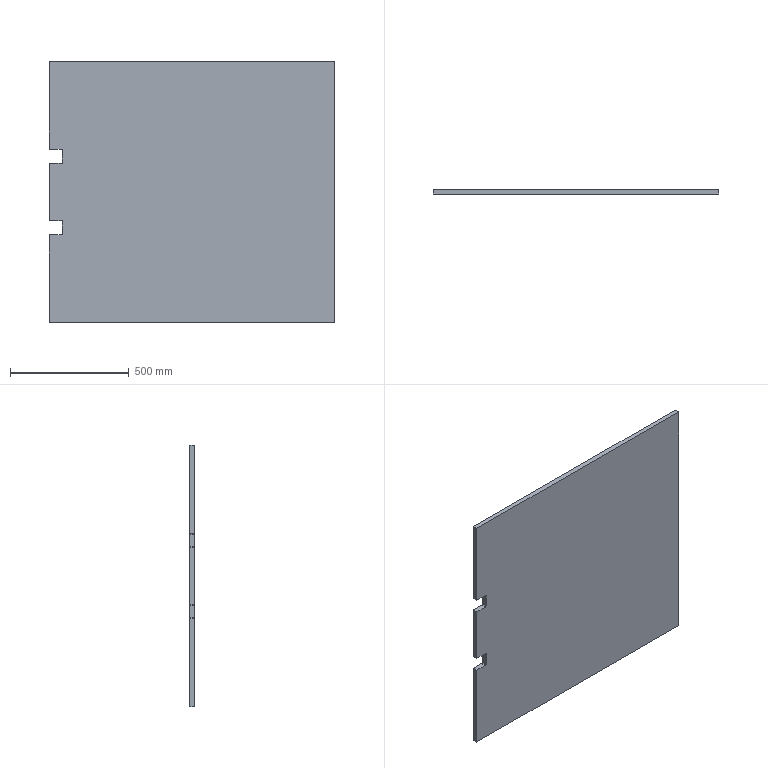Part | STEP file | A14-004 | 1 solid | 18 faces | box 1200 x 20 x 1100 mm | volume 26268429 mm3 | plane 14 | cylinder 4 | commonest cylinder face diameters 10 x4
STEP:
#1=CARTESIAN_POINT('',(0.,0.,0.));
#2=DIRECTION('',(0.,0.,1.));
#3=DIRECTION('',(1.,0.,0.));
#4=AXIS2_PLACEMENT_3D('',#1,#2,#3);
#5=CARTESIAN_POINT('',(-600.,0.,-120.));
#6=VERTEX_POINT('',#5);
#7=CARTESIAN_POINT('',(-600.,0.,120.));
#8=VERTEX_POINT('',#7);
#9=CARTESIAN_POINT('',(-600.,0.,-550.));
#10=DIRECTION('',(0.,0.,1.));
#11=VECTOR('',#10,1.);
#12=LINE('',#9,#11);
#13=CARTESIAN_POINT('',(-600.,20.,-550.));
#14=DIRECTION('',(1.,0.,0.));
#15=DIRECTION('',(0.,0.,-1.));
#16=AXIS2_PLACEMENT_3D('',#13,#14,#15);
#17=PLANE('',#16);
#18=CARTESIAN_POINT('',(0.,-20.));
#19=DIRECTION('',(-1.,0.));
#20=VECTOR('',#19,1.);
#21=LINE('',#18,#20);
#22=(GEOMETRIC_REPRESENTATION_CONTEXT(2)PARAMETRIC_REPRESENTATION_CONTEXT()REPRESENTATION_CONTEXT('',''));
#23=DEFINITIONAL_REPRESENTATION('',(#21),#22);
#24=PCURVE('',#17,#23);
#25=CARTESIAN_POINT('',(0.,0.,0.));
#26=DIRECTION('',(0.,1.,0.));
#27=DIRECTION('',(0.,0.,1.));
#28=AXIS2_PLACEMENT_3D('',#25,#26,#27);
#29=PLANE('',#28);
#30=CARTESIAN_POINT('',(-550.,-600.));
#31=DIRECTION('',(1.,0.));
#32=VECTOR('',#31,1.);
#33=LINE('',#30,#32);
#34=(GEOMETRIC_REPRESENTATION_CONTEXT(2)PARAMETRIC_REPRESENTATION_CONTEXT()REPRESENTATION_CONTEXT('',''));
#35=DEFINITIONAL_REPRESENTATION('',(#33),#34);
#36=PCURVE('',#29,#35);
#37=SURFACE_CURVE('',#12,(#24,#36),.PCURVE_S1.);
#38=EDGE_CURVE('',#6,#8,#37,.T.);
#39=ORIENTED_EDGE('',*,*,#38,.T.);
#40=CARTESIAN_POINT('',(-600.,20.,120.));
#41=VERTEX_POINT('',#40);
#42=CARTESIAN_POINT('',(-600.,0.,120.));
#43=DIRECTION('',(0.,1.,0.));
#44=VECTOR('',#43,1.);
#45=LINE('',#42,#44);
#46=CARTESIAN_POINT('',(-670.,-20.));
#47=DIRECTION('',(0.,1.));
#48=VECTOR('',#47,1.);
#49=LINE('',#46,#48);
#50=(GEOMETRIC_REPRESENTATION_CONTEXT(2)PARAMETRIC_REPRESENTATION_CONTEXT()REPRESENTATION_CONTEXT('',''));
#51=DEFINITIONAL_REPRESENTATION('',(#49),#50);
#52=PCURVE('',#17,#51);
#53=CARTESIAN_POINT('',(-600.,0.,120.));
#54=DIRECTION('',(0.,0.,-1.));
#55=DIRECTION('',(-1.,0.,0.));
#56=AXIS2_PLACEMENT_3D('',#53,#54,#55);
#57=PLANE('',#56);
#58=CARTESIAN_POINT('',(0.,0.));
#59=DIRECTION('',(0.,1.));
#60=VECTOR('',#59,1.);
#61=LINE('',#58,#60);
#62=(GEOMETRIC_REPRESENTATION_CONTEXT(2)PARAMETRIC_REPRESENTATION_CONTEXT()REPRESENTATION_CONTEXT('',''));
#63=DEFINITIONAL_REPRESENTATION('',(#61),#62);
#64=PCURVE('',#57,#63);
#65=SURFACE_CURVE('',#45,(#52,#64),.PCURVE_S1.);
#66=EDGE_CURVE('',#8,#41,#65,.T.);
#67=ORIENTED_EDGE('',*,*,#66,.T.);
#68=CARTESIAN_POINT('',(-600.,20.,-120.));
#69=VERTEX_POINT('',#68);
#70=CARTESIAN_POINT('',(-600.,20.,-550.));
#71=DIRECTION('',(0.,0.,1.));
#72=VECTOR('',#71,1.);
#73=LINE('',#70,#72);
#74=CARTESIAN_POINT('',(0.,0.));
#75=DIRECTION('',(-1.,0.));
#76=VECTOR('',#75,1.);
#77=LINE('',#74,#76);
#78=(GEOMETRIC_REPRESENTATION_CONTEXT(2)PARAMETRIC_REPRESENTATION_CONTEXT()REPRESENTATION_CONTEXT('',''));
#79=DEFINITIONAL_REPRESENTATION('',(#77),#78);
#80=PCURVE('',#17,#79);
#81=CARTESIAN_POINT('',(0.,20.,0.));
#82=DIRECTION('',(0.,1.,0.));
#83=DIRECTION('',(0.,0.,1.));
#84=AXIS2_PLACEMENT_3D('',#81,#82,#83);
#85=PLANE('',#84);
#86=CARTESIAN_POINT('',(-550.,-600.));
#87=DIRECTION('',(1.,0.));
#88=VECTOR('',#87,1.);
#89=LINE('',#86,#88);
#90=(GEOMETRIC_REPRESENTATION_CONTEXT(2)PARAMETRIC_REPRESENTATION_CONTEXT()REPRESENTATION_CONTEXT('',''));
#91=DEFINITIONAL_REPRESENTATION('',(#89),#90);
#92=PCURVE('',#85,#91);
#93=SURFACE_CURVE('',#73,(#80,#92),.PCURVE_S1.);
#94=EDGE_CURVE('',#69,#41,#93,.T.);
#95=ORIENTED_EDGE('',*,*,#94,.F.);
#96=CARTESIAN_POINT('',(-600.,0.,-120.));
#97=DIRECTION('',(0.,1.,0.));
#98=VECTOR('',#97,1.);
#99=LINE('',#96,#98);
#100=CARTESIAN_POINT('',(-430.,-20.));
#101=DIRECTION('',(0.,1.));
#102=VECTOR('',#101,1.);
#103=LINE('',#100,#102);
#104=(GEOMETRIC_REPRESENTATION_CONTEXT(2)PARAMETRIC_REPRESENTATION_CONTEXT()REPRESENTATION_CONTEXT('',''));
#105=DEFINITIONAL_REPRESENTATION('',(#103),#104);
#106=PCURVE('',#17,#105);
#107=CARTESIAN_POINT('',(-600.,0.,-120.));
#108=DIRECTION('',(0.,0.,1.));
#109=DIRECTION('',(1.,0.,0.));
#110=AXIS2_PLACEMENT_3D('',#107,#108,#109);
#111=PLANE('',#110);
#112=CARTESIAN_POINT('',(0.,0.));
#113=DIRECTION('',(0.,1.));
#114=VECTOR('',#113,1.);
#115=LINE('',#112,#114);
#116=(GEOMETRIC_REPRESENTATION_CONTEXT(2)PARAMETRIC_REPRESENTATION_CONTEXT()REPRESENTATION_CONTEXT('',''));
#117=DEFINITIONAL_REPRESENTATION('',(#115),#116);
#118=PCURVE('',#111,#117);
#119=SURFACE_CURVE('',#99,(#106,#118),.PCURVE_S1.);
#120=EDGE_CURVE('',#6,#69,#119,.T.);
#121=ORIENTED_EDGE('',*,*,#120,.F.);
#122=EDGE_LOOP('',(#39,#67,#95,#121));
#123=FACE_BOUND('',#122,.T.);
#124=ADVANCED_FACE('',(#123),#17,.F.);
#125=CARTESIAN_POINT('',(-600.,0.,-550.));
#126=VERTEX_POINT('',#125);
#127=CARTESIAN_POINT('',(-600.,0.,-180.));
#128=VERTEX_POINT('',#127);
#129=CARTESIAN_POINT('',(-600.,0.,-550.));
#130=DIRECTION('',(0.,0.,1.));
#131=VECTOR('',#130,1.);
#132=LINE('',#129,#131);
#133=CARTESIAN_POINT('',(-600.,20.,-550.));
#134=DIRECTION('',(1.,0.,0.));
#135=DIRECTION('',(0.,0.,-1.));
#136=AXIS2_PLACEMENT_3D('',#133,#134,#135);
#137=PLANE('',#136);
#138=CARTESIAN_POINT('',(0.,-20.));
#139=DIRECTION('',(-1.,0.));
#140=VECTOR('',#139,1.);
#141=LINE('',#138,#140);
#142=(GEOMETRIC_REPRESENTATION_CONTEXT(2)PARAMETRIC_REPRESENTATION_CONTEXT()REPRESENTATION_CONTEXT('',''));
#143=DEFINITIONAL_REPRESENTATION('',(#141),#142);
#144=PCURVE('',#137,#143);
#145=CARTESIAN_POINT('',(-550.,-600.));
#146=DIRECTION('',(1.,0.));
#147=VECTOR('',#146,1.);
#148=LINE('',#145,#147);
#149=(GEOMETRIC_REPRESENTATION_CONTEXT(2)PARAMETRIC_REPRESENTATION_CONTEXT()REPRESENTATION_CONTEXT('',''));
#150=DEFINITIONAL_REPRESENTATION('',(#148),#149);
#151=PCURVE('',#29,#150);
#152=SURFACE_CURVE('',#132,(#144,#151),.PCURVE_S1.);
#153=EDGE_CURVE('',#126,#128,#152,.T.);
#154=ORIENTED_EDGE('',*,*,#153,.T.);
#155=CARTESIAN_POINT('',(-600.,20.,-180.));
#156=VERTEX_POINT('',#155);
#157=CARTESIAN_POINT('',(-600.,0.,-180.));
#158=DIRECTION('',(0.,1.,0.));
#159=VECTOR('',#158,1.);
#160=LINE('',#157,#159);
#161=CARTESIAN_POINT('',(-370.,-20.));
#162=DIRECTION('',(0.,1.));
#163=VECTOR('',#162,1.);
#164=LINE('',#161,#163);
#165=(GEOMETRIC_REPRESENTATION_CONTEXT(2)PARAMETRIC_REPRESENTATION_CONTEXT()REPRESENTATION_CONTEXT('',''));
#166=DEFINITIONAL_REPRESENTATION('',(#164),#165);
#167=PCURVE('',#137,#166);
#168=CARTESIAN_POINT('',(-600.,0.,-180.));
#169=DIRECTION('',(0.,0.,-1.));
#170=DIRECTION('',(-1.,0.,0.));
#171=AXIS2_PLACEMENT_3D('',#168,#169,#170);
#172=PLANE('',#171);
#173=CARTESIAN_POINT('',(0.,0.));
#174=DIRECTION('',(0.,1.));
#175=VECTOR('',#174,1.);
#176=LINE('',#173,#175);
#177=(GEOMETRIC_REPRESENTATION_CONTEXT(2)PARAMETRIC_REPRESENTATION_CONTEXT()REPRESENTATION_CONTEXT('',''));
#178=DEFINITIONAL_REPRESENTATION('',(#176),#177);
#179=PCURVE('',#172,#178);
#180=SURFACE_CURVE('',#160,(#167,#179),.PCURVE_S1.);
#181=EDGE_CURVE('',#128,#156,#180,.T.);
#182=ORIENTED_EDGE('',*,*,#181,.T.);
#183=CARTESIAN_POINT('',(-600.,20.,-550.));
#184=VERTEX_POINT('',#183);
#185=CARTESIAN_POINT('',(-600.,20.,-550.));
#186=DIRECTION('',(0.,0.,1.));
#187=VECTOR('',#186,1.);
#188=LINE('',#185,#187);
#189=CARTESIAN_POINT('',(0.,0.));
#190=DIRECTION('',(-1.,0.));
#191=VECTOR('',#190,1.);
#192=LINE('',#189,#191);
#193=(GEOMETRIC_REPRESENTATION_CONTEXT(2)PARAMETRIC_REPRESENTATION_CONTEXT()REPRESENTATION_CONTEXT('',''));
#194=DEFINITIONAL_REPRESENTATION('',(#192),#193);
#195=PCURVE('',#137,#194);
#196=CARTESIAN_POINT('',(-550.,-600.));
#197=DIRECTION('',(1.,0.));
#198=VECTOR('',#197,1.);
#199=LINE('',#196,#198);
#200=(GEOMETRIC_REPRESENTATION_CONTEXT(2)PARAMETRIC_REPRESENTATION_CONTEXT()REPRESENTATION_CONTEXT('',''));
#201=DEFINITIONAL_REPRESENTATION('',(#199),#200);
#202=PCURVE('',#85,#201);
#203=SURFACE_CURVE('',#188,(#195,#202),.PCURVE_S1.);
#204=EDGE_CURVE('',#184,#156,#203,.T.);
#205=ORIENTED_EDGE('',*,*,#204,.F.);
#206=CARTESIAN_POINT('',(-600.,20.,-550.));
#207=DIRECTION('',(0.,-1.,0.));
#208=VECTOR('',#207,1.);
#209=LINE('',#206,#208);
#210=CARTESIAN_POINT('',(0.,0.));
#211=DIRECTION('',(0.,-1.));
#212=VECTOR('',#211,1.);
#213=LINE('',#210,#212);
#214=(GEOMETRIC_REPRESENTATION_CONTEXT(2)PARAMETRIC_REPRESENTATION_CONTEXT()REPRESENTATION_CONTEXT('',''));
#215=DEFINITIONAL_REPRESENTATION('',(#213),#214);
#216=PCURVE('',#137,#215);
#217=CARTESIAN_POINT('',(-600.,20.,-550.));
#218=DIRECTION('',(0.,0.,1.));
#219=DIRECTION('',(1.,0.,0.));
#220=AXIS2_PLACEMENT_3D('',#217,#218,#219);
#221=PLANE('',#220);
#222=CARTESIAN_POINT('',(0.,0.));
#223=DIRECTION('',(0.,-1.));
#224=VECTOR('',#223,1.);
#225=LINE('',#222,#224);
#226=(GEOMETRIC_REPRESENTATION_CONTEXT(2)PARAMETRIC_REPRESENTATION_CONTEXT()REPRESENTATION_CONTEXT('',''));
#227=DEFINITIONAL_REPRESENTATION('',(#225),#226);
#228=PCURVE('',#221,#227);
#229=SURFACE_CURVE('',#209,(#216,#228),.PCURVE_S1.);
#230=EDGE_CURVE('',#184,#126,#229,.T.);
#231=ORIENTED_EDGE('',*,*,#230,.T.);
#232=EDGE_LOOP('',(#154,#182,#205,#231));
#233=FACE_BOUND('',#232,.T.);
#234=ADVANCED_FACE('',(#233),#137,.F.);
#235=CARTESIAN_POINT('',(600.,0.,550.));
#236=VERTEX_POINT('',#235);
#237=CARTESIAN_POINT('',(600.,0.,-550.));
#238=VERTEX_POINT('',#237);
#239=CARTESIAN_POINT('',(600.,0.,-550.));
#240=DIRECTION('',(0.,0.,-1.));
#241=VECTOR('',#240,1.);
#242=LINE('',#239,#241);
#243=CARTESIAN_POINT('',(600.,20.,-550.));
#244=DIRECTION('',(-1.,0.,0.));
#245=DIRECTION('',(0.,0.,1.));
#246=AXIS2_PLACEMENT_3D('',#243,#244,#245);
#247=PLANE('',#246);
#248=CARTESIAN_POINT('',(0.,-20.));
#249=DIRECTION('',(-1.,0.));
#250=VECTOR('',#249,1.);
#251=LINE('',#248,#250);
#252=(GEOMETRIC_REPRESENTATION_CONTEXT(2)PARAMETRIC_REPRESENTATION_CONTEXT()REPRESENTATION_CONTEXT('',''));
#253=DEFINITIONAL_REPRESENTATION('',(#251),#252);
#254=PCURVE('',#247,#253);
#255=CARTESIAN_POINT('',(-550.,600.));
#256=DIRECTION('',(-1.,0.));
#257=VECTOR('',#256,1.);
#258=LINE('',#255,#257);
#259=(GEOMETRIC_REPRESENTATION_CONTEXT(2)PARAMETRIC_REPRESENTATION_CONTEXT()REPRESENTATION_CONTEXT('',''));
#260=DEFINITIONAL_REPRESENTATION('',(#258),#259);
#261=PCURVE('',#29,#260);
#262=SURFACE_CURVE('',#242,(#254,#261),.PCURVE_S1.);
#263=EDGE_CURVE('',#236,#238,#262,.T.);
#264=ORIENTED_EDGE('',*,*,#263,.T.);
#265=CARTESIAN_POINT('',(600.,20.,-550.));
#266=VERTEX_POINT('',#265);
#267=CARTESIAN_POINT('',(600.,20.,-550.));
#268=DIRECTION('',(0.,-1.,0.));
#269=VECTOR('',#268,1.);
#270=LINE('',#267,#269);
#271=CARTESIAN_POINT('',(0.,0.));
#272=DIRECTION('',(0.,-1.));
#273=VECTOR('',#272,1.);
#274=LINE('',#271,#273);
#275=(GEOMETRIC_REPRESENTATION_CONTEXT(2)PARAMETRIC_REPRESENTATION_CONTEXT()REPRESENTATION_CONTEXT('',''));
#276=DEFINITIONAL_REPRESENTATION('',(#274),#275);
#277=PCURVE('',#247,#276);
#278=CARTESIAN_POINT('',(1200.,0.));
#279=DIRECTION('',(0.,-1.));
#280=VECTOR('',#279,1.);
#281=LINE('',#278,#280);
#282=(GEOMETRIC_REPRESENTATION_CONTEXT(2)PARAMETRIC_REPRESENTATION_CONTEXT()REPRESENTATION_CONTEXT('',''));
#283=DEFINITIONAL_REPRESENTATION('',(#281),#282);
#284=PCURVE('',#221,#283);
#285=SURFACE_CURVE('',#270,(#277,#284),.PCURVE_S1.);
#286=EDGE_CURVE('',#266,#238,#285,.T.);
#287=ORIENTED_EDGE('',*,*,#286,.F.);
#288=CARTESIAN_POINT('',(600.,20.,550.));
#289=VERTEX_POINT('',#288);
#290=CARTESIAN_POINT('',(600.,20.,-550.));
#291=DIRECTION('',(0.,0.,-1.));
#292=VECTOR('',#291,1.);
#293=LINE('',#290,#292);
#294=CARTESIAN_POINT('',(0.,0.));
#295=DIRECTION('',(-1.,0.));
#296=VECTOR('',#295,1.);
#297=LINE('',#294,#296);
#298=(GEOMETRIC_REPRESENTATION_CONTEXT(2)PARAMETRIC_REPRESENTATION_CONTEXT()REPRESENTATION_CONTEXT('',''));
#299=DEFINITIONAL_REPRESENTATION('',(#297),#298);
#300=PCURVE('',#247,#299);
#301=CARTESIAN_POINT('',(-550.,600.));
#302=DIRECTION('',(-1.,0.));
#303=VECTOR('',#302,1.);
#304=LINE('',#301,#303);
#305=(GEOMETRIC_REPRESENTATION_CONTEXT(2)PARAMETRIC_REPRESENTATION_CONTEXT()REPRESENTATION_CONTEXT('',''));
#306=DEFINITIONAL_REPRESENTATION('',(#304),#305);
#307=PCURVE('',#85,#306);
#308=SURFACE_CURVE('',#293,(#300,#307),.PCURVE_S1.);
#309=EDGE_CURVE('',#289,#266,#308,.T.);
#310=ORIENTED_EDGE('',*,*,#309,.F.);
#311=CARTESIAN_POINT('',(600.,20.,550.));
#312=DIRECTION('',(0.,-1.,0.));
#313=VECTOR('',#312,1.);
#314=LINE('',#311,#313);
#315=CARTESIAN_POINT('',(1100.,0.));
#316=DIRECTION('',(0.,-1.));
#317=VECTOR('',#316,1.);
#318=LINE('',#315,#317);
#319=(GEOMETRIC_REPRESENTATION_CONTEXT(2)PARAMETRIC_REPRESENTATION_CONTEXT()REPRESENTATION_CONTEXT('',''));
#320=DEFINITIONAL_REPRESENTATION('',(#318),#319);
#321=PCURVE('',#247,#320);
#322=CARTESIAN_POINT('',(-600.,20.,550.));
#323=DIRECTION('',(0.,0.,-1.));
#324=DIRECTION('',(-1.,0.,0.));
#325=AXIS2_PLACEMENT_3D('',#322,#323,#324);
#326=PLANE('',#325);
#327=CARTESIAN_POINT('',(-1200.,0.));
#328=DIRECTION('',(0.,-1.));
#329=VECTOR('',#328,1.);
#330=LINE('',#327,#329);
#331=(GEOMETRIC_REPRESENTATION_CONTEXT(2)PARAMETRIC_REPRESENTATION_CONTEXT()REPRESENTATION_CONTEXT('',''));
#332=DEFINITIONAL_REPRESENTATION('',(#330),#331);
#333=PCURVE('',#326,#332);
#334=SURFACE_CURVE('',#314,(#321,#333),.PCURVE_S1.);
#335=EDGE_CURVE('',#289,#236,#334,.T.);
#336=ORIENTED_EDGE('',*,*,#335,.T.);
#337=EDGE_LOOP('',(#264,#287,#310,#336));
#338=FACE_BOUND('',#337,.T.);
#339=ADVANCED_FACE('',(#338),#247,.F.);
#340=CARTESIAN_POINT('',(-600.,0.,-550.));
#341=DIRECTION('',(-1.,0.,0.));
#342=VECTOR('',#341,1.);
#343=LINE('',#340,#342);
#344=CARTESIAN_POINT('',(0.,-20.));
#345=DIRECTION('',(-1.,0.));
#346=VECTOR('',#345,1.);
#347=LINE('',#344,#346);
#348=(GEOMETRIC_REPRESENTATION_CONTEXT(2)PARAMETRIC_REPRESENTATION_CONTEXT()REPRESENTATION_CONTEXT('',''));
#349=DEFINITIONAL_REPRESENTATION('',(#347),#348);
#350=PCURVE('',#221,#349);
#351=CARTESIAN_POINT('',(-550.,-600.));
#352=DIRECTION('',(0.,-1.));
#353=VECTOR('',#352,1.);
#354=LINE('',#351,#353);
#355=(GEOMETRIC_REPRESENTATION_CONTEXT(2)PARAMETRIC_REPRESENTATION_CONTEXT()REPRESENTATION_CONTEXT('',''));
#356=DEFINITIONAL_REPRESENTATION('',(#354),#355);
#357=PCURVE('',#29,#356);
#358=SURFACE_CURVE('',#343,(#350,#357),.PCURVE_S1.);
#359=EDGE_CURVE('',#238,#126,#358,.T.);
#360=ORIENTED_EDGE('',*,*,#359,.T.);
#361=ORIENTED_EDGE('',*,*,#230,.F.);
#362=CARTESIAN_POINT('',(-600.,20.,-550.));
#363=DIRECTION('',(-1.,0.,0.));
#364=VECTOR('',#363,1.);
#365=LINE('',#362,#364);
#366=CARTESIAN_POINT('',(0.,0.));
#367=DIRECTION('',(-1.,0.));
#368=VECTOR('',#367,1.);
#369=LINE('',#366,#368);
#370=(GEOMETRIC_REPRESENTATION_CONTEXT(2)PARAMETRIC_REPRESENTATION_CONTEXT()REPRESENTATION_CONTEXT('',''));
#371=DEFINITIONAL_REPRESENTATION('',(#369),#370);
#372=PCURVE('',#221,#371);
#373=CARTESIAN_POINT('',(-550.,-600.));
#374=DIRECTION('',(0.,-1.));
#375=VECTOR('',#374,1.);
#376=LINE('',#373,#375);
#377=(GEOMETRIC_REPRESENTATION_CONTEXT(2)PARAMETRIC_REPRESENTATION_CONTEXT()REPRESENTATION_CONTEXT('',''));
#378=DEFINITIONAL_REPRESENTATION('',(#376),#377);
#379=PCURVE('',#85,#378);
#380=SURFACE_CURVE('',#365,(#372,#379),.PCURVE_S1.);
#381=EDGE_CURVE('',#266,#184,#380,.T.);
#382=ORIENTED_EDGE('',*,*,#381,.F.);
#383=ORIENTED_EDGE('',*,*,#286,.T.);
#384=EDGE_LOOP('',(#360,#361,#382,#383));
#385=FACE_BOUND('',#384,.T.);
#386=ADVANCED_FACE('',(#385),#221,.F.);
#387=CARTESIAN_POINT('',(-600.,20.,180.));
#388=VERTEX_POINT('',#387);
#389=CARTESIAN_POINT('',(-600.,20.,550.));
#390=VERTEX_POINT('',#389);
#391=CARTESIAN_POINT('',(-600.,20.,-550.));
#392=DIRECTION('',(0.,0.,1.));
#393=VECTOR('',#392,1.);
#394=LINE('',#391,#393);
#395=CARTESIAN_POINT('',(-600.,20.,-550.));
#396=DIRECTION('',(1.,0.,0.));
#397=DIRECTION('',(0.,0.,-1.));
#398=AXIS2_PLACEMENT_3D('',#395,#396,#397);
#399=PLANE('',#398);
#400=CARTESIAN_POINT('',(0.,0.));
#401=DIRECTION('',(-1.,0.));
#402=VECTOR('',#401,1.);
#403=LINE('',#400,#402);
#404=(GEOMETRIC_REPRESENTATION_CONTEXT(2)PARAMETRIC_REPRESENTATION_CONTEXT()REPRESENTATION_CONTEXT('',''));
#405=DEFINITIONAL_REPRESENTATION('',(#403),#404);
#406=PCURVE('',#399,#405);
#407=CARTESIAN_POINT('',(-550.,-600.));
#408=DIRECTION('',(1.,0.));
#409=VECTOR('',#408,1.);
#410=LINE('',#407,#409);
#411=(GEOMETRIC_REPRESENTATION_CONTEXT(2)PARAMETRIC_REPRESENTATION_CONTEXT()REPRESENTATION_CONTEXT('',''));
#412=DEFINITIONAL_REPRESENTATION('',(#410),#411);
#413=PCURVE('',#85,#412);
#414=SURFACE_CURVE('',#394,(#406,#413),.PCURVE_S1.);
#415=EDGE_CURVE('',#388,#390,#414,.T.);
#416=ORIENTED_EDGE('',*,*,#415,.F.);
#417=CARTESIAN_POINT('',(-600.,0.,180.));
#418=VERTEX_POINT('',#417);
#419=CARTESIAN_POINT('',(-600.,0.,180.));
#420=DIRECTION('',(0.,1.,0.));
#421=VECTOR('',#420,1.);
#422=LINE('',#419,#421);
#423=CARTESIAN_POINT('',(-730.,-20.));
#424=DIRECTION('',(0.,1.));
#425=VECTOR('',#424,1.);
#426=LINE('',#423,#425);
#427=(GEOMETRIC_REPRESENTATION_CONTEXT(2)PARAMETRIC_REPRESENTATION_CONTEXT()REPRESENTATION_CONTEXT('',''));
#428=DEFINITIONAL_REPRESENTATION('',(#426),#427);
#429=PCURVE('',#399,#428);
#430=CARTESIAN_POINT('',(-600.,0.,180.));
#431=DIRECTION('',(0.,0.,1.));
#432=DIRECTION('',(1.,0.,0.));
#433=AXIS2_PLACEMENT_3D('',#430,#431,#432);
#434=PLANE('',#433);
#435=CARTESIAN_POINT('',(0.,0.));
#436=DIRECTION('',(0.,1.));
#437=VECTOR('',#436,1.);
#438=LINE('',#435,#437);
#439=(GEOMETRIC_REPRESENTATION_CONTEXT(2)PARAMETRIC_REPRESENTATION_CONTEXT()REPRESENTATION_CONTEXT('',''));
#440=DEFINITIONAL_REPRESENTATION('',(#438),#439);
#441=PCURVE('',#434,#440);
#442=SURFACE_CURVE('',#422,(#429,#441),.PCURVE_S1.);
#443=EDGE_CURVE('',#418,#388,#442,.T.);
#444=ORIENTED_EDGE('',*,*,#443,.F.);
#445=CARTESIAN_POINT('',(-600.,0.,550.));
#446=VERTEX_POINT('',#445);
#447=CARTESIAN_POINT('',(-600.,0.,-550.));
#448=DIRECTION('',(0.,0.,1.));
#449=VECTOR('',#448,1.);
#450=LINE('',#447,#449);
#451=CARTESIAN_POINT('',(0.,-20.));
#452=DIRECTION('',(-1.,0.));
#453=VECTOR('',#452,1.);
#454=LINE('',#451,#453);
#455=(GEOMETRIC_REPRESENTATION_CONTEXT(2)PARAMETRIC_REPRESENTATION_CONTEXT()REPRESENTATION_CONTEXT('',''));
#456=DEFINITIONAL_REPRESENTATION('',(#454),#455);
#457=PCURVE('',#399,#456);
#458=CARTESIAN_POINT('',(-550.,-600.));
#459=DIRECTION('',(1.,0.));
#460=VECTOR('',#459,1.);
#461=LINE('',#458,#460);
#462=(GEOMETRIC_REPRESENTATION_CONTEXT(2)PARAMETRIC_REPRESENTATION_CONTEXT()REPRESENTATION_CONTEXT('',''));
#463=DEFINITIONAL_REPRESENTATION('',(#461),#462);
#464=PCURVE('',#29,#463);
#465=SURFACE_CURVE('',#450,(#457,#464),.PCURVE_S1.);
#466=EDGE_CURVE('',#418,#446,#465,.T.);
#467=ORIENTED_EDGE('',*,*,#466,.T.);
#468=CARTESIAN_POINT('',(-600.,20.,550.));
#469=DIRECTION('',(0.,-1.,0.));
#470=VECTOR('',#469,1.);
#471=LINE('',#468,#470);
#472=CARTESIAN_POINT('',(-1100.,0.));
#473=DIRECTION('',(0.,-1.));
#474=VECTOR('',#473,1.);
#475=LINE('',#472,#474);
#476=(GEOMETRIC_REPRESENTATION_CONTEXT(2)PARAMETRIC_REPRESENTATION_CONTEXT()REPRESENTATION_CONTEXT('',''));
#477=DEFINITIONAL_REPRESENTATION('',(#475),#476);
#478=PCURVE('',#399,#477);
#479=CARTESIAN_POINT('',(0.,0.));
#480=DIRECTION('',(0.,-1.));
#481=VECTOR('',#480,1.);
#482=LINE('',#479,#481);
#483=(GEOMETRIC_REPRESENTATION_CONTEXT(2)PARAMETRIC_REPRESENTATION_CONTEXT()REPRESENTATION_CONTEXT('',''));
#484=DEFINITIONAL_REPRESENTATION('',(#482),#483);
#485=PCURVE('',#326,#484);
#486=SURFACE_CURVE('',#471,(#478,#485),.PCURVE_S1.);
#487=EDGE_CURVE('',#390,#446,#486,.T.);
#488=ORIENTED_EDGE('',*,*,#487,.F.);
#489=EDGE_LOOP('',(#416,#444,#467,#488));
#490=FACE_BOUND('',#489,.T.);
#491=ADVANCED_FACE('',(#490),#399,.F.);
#492=CARTESIAN_POINT('',(-600.,0.,550.));
#493=DIRECTION('',(1.,0.,0.));
#494=VECTOR('',#493,1.);
#495=LINE('',#492,#494);
#496=CARTESIAN_POINT('',(0.,-20.));
#497=DIRECTION('',(-1.,0.));
#498=VECTOR('',#497,1.);
#499=LINE('',#496,#498);
#500=(GEOMETRIC_REPRESENTATION_CONTEXT(2)PARAMETRIC_REPRESENTATION_CONTEXT()REPRESENTATION_CONTEXT('',''));
#501=DEFINITIONAL_REPRESENTATION('',(#499),#500);
#502=PCURVE('',#326,#501);
#503=CARTESIAN_POINT('',(550.,-600.));
#504=DIRECTION('',(0.,1.));
#505=VECTOR('',#504,1.);
#506=LINE('',#503,#505);
#507=(GEOMETRIC_REPRESENTATION_CONTEXT(2)PARAMETRIC_REPRESENTATION_CONTEXT()REPRESENTATION_CONTEXT('',''));
#508=DEFINITIONAL_REPRESENTATION('',(#506),#507);
#509=PCURVE('',#29,#508);
#510=SURFACE_CURVE('',#495,(#502,#509),.PCURVE_S1.);
#511=EDGE_CURVE('',#446,#236,#510,.T.);
#512=ORIENTED_EDGE('',*,*,#511,.T.);
#513=ORIENTED_EDGE('',*,*,#335,.F.);
#514=CARTESIAN_POINT('',(-600.,20.,550.));
#515=DIRECTION('',(1.,0.,0.));
#516=VECTOR('',#515,1.);
#517=LINE('',#514,#516);
#518=CARTESIAN_POINT('',(0.,0.));
#519=DIRECTION('',(-1.,0.));
#520=VECTOR('',#519,1.);
#521=LINE('',#518,#520);
#522=(GEOMETRIC_REPRESENTATION_CONTEXT(2)PARAMETRIC_REPRESENTATION_CONTEXT()REPRESENTATION_CONTEXT('',''));
#523=DEFINITIONAL_REPRESENTATION('',(#521),#522);
#524=PCURVE('',#326,#523);
#525=CARTESIAN_POINT('',(550.,-600.));
#526=DIRECTION('',(0.,1.));
#527=VECTOR('',#526,1.);
#528=LINE('',#525,#527);
#529=(GEOMETRIC_REPRESENTATION_CONTEXT(2)PARAMETRIC_REPRESENTATION_CONTEXT()REPRESENTATION_CONTEXT('',''));
#530=DEFINITIONAL_REPRESENTATION('',(#528),#529);
#531=PCURVE('',#85,#530);
#532=SURFACE_CURVE('',#517,(#524,#531),.PCURVE_S1.);
#533=EDGE_CURVE('',#390,#289,#532,.T.);
#534=ORIENTED_EDGE('',*,*,#533,.F.);
#535=ORIENTED_EDGE('',*,*,#487,.T.);
#536=EDGE_LOOP('',(#512,#513,#534,#535));
#537=FACE_BOUND('',#536,.T.);
#538=ADVANCED_FACE('',(#537),#326,.F.);
#539=CARTESIAN_POINT('',(-550.,20.,120.));
#540=VERTEX_POINT('',#539);
#541=CARTESIAN_POINT('',(-600.,20.,120.));
#542=DIRECTION('',(-1.,0.,0.));
#543=VECTOR('',#542,1.);
#544=LINE('',#541,#543);
#545=CARTESIAN_POINT('',(120.,-600.));
#546=DIRECTION('',(0.,-1.));
#547=VECTOR('',#546,1.);
#548=LINE('',#545,#547);
#549=(GEOMETRIC_REPRESENTATION_CONTEXT(2)PARAMETRIC_REPRESENTATION_CONTEXT()REPRESENTATION_CONTEXT('',''));
#550=DEFINITIONAL_REPRESENTATION('',(#548),#549);
#551=PCURVE('',#85,#550);
#552=CARTESIAN_POINT('',(0.,20.));
#553=DIRECTION('',(1.,0.));
#554=VECTOR('',#553,1.);
#555=LINE('',#552,#554);
#556=(GEOMETRIC_REPRESENTATION_CONTEXT(2)PARAMETRIC_REPRESENTATION_CONTEXT()REPRESENTATION_CONTEXT('',''));
#557=DEFINITIONAL_REPRESENTATION('',(#555),#556);
#558=PCURVE('',#57,#557);
#559=SURFACE_CURVE('',#544,(#551,#558),.PCURVE_S1.);
#560=EDGE_CURVE('',#540,#41,#559,.T.);
#561=ORIENTED_EDGE('',*,*,#560,.F.);
#562=CARTESIAN_POINT('',(-545.,20.,125.));
#563=VERTEX_POINT('',#562);
#564=CARTESIAN_POINT('',(-550.,20.,125.));
#565=DIRECTION('',(0.,1.,0.));
#566=DIRECTION('',(0.,0.,-1.));
#567=AXIS2_PLACEMENT_3D('',#564,#565,#566);
#568=CIRCLE('',#567,5.);
#569=CARTESIAN_POINT('',(125.,-550.));
#570=DIRECTION('',(-1.,0.));
#571=AXIS2_PLACEMENT_2D('',#569,#570);
#572=CIRCLE('',#571,5.);
#573=(GEOMETRIC_REPRESENTATION_CONTEXT(2)PARAMETRIC_REPRESENTATION_CONTEXT()REPRESENTATION_CONTEXT('',''));
#574=DEFINITIONAL_REPRESENTATION('',(#572),#573);
#575=PCURVE('',#85,#574);
#576=CARTESIAN_POINT('',(-550.,0.,125.));
#577=DIRECTION('',(0.,1.,0.));
#578=DIRECTION('',(0.,0.,1.));
#579=AXIS2_PLACEMENT_3D('',#576,#577,#578);
#580=CYLINDRICAL_SURFACE('',#579,5.);
#581=CARTESIAN_POINT('',(-3.142,20.));
#582=DIRECTION('',(1.,0.));
#583=VECTOR('',#582,1.);
#584=LINE('',#581,#583);
#585=(GEOMETRIC_REPRESENTATION_CONTEXT(2)PARAMETRIC_REPRESENTATION_CONTEXT()REPRESENTATION_CONTEXT('',''));
#586=DEFINITIONAL_REPRESENTATION('',(#584),#585);
#587=PCURVE('',#580,#586);
#588=SURFACE_CURVE('',#568,(#575,#587),.PCURVE_S1.);
#589=EDGE_CURVE('',#563,#540,#588,.T.);
#590=ORIENTED_EDGE('',*,*,#589,.F.);
#591=CARTESIAN_POINT('',(-545.,20.,175.));
#592=VERTEX_POINT('',#591);
#593=CARTESIAN_POINT('',(-545.,20.,175.));
#594=DIRECTION('',(0.,0.,-1.));
#595=VECTOR('',#594,1.);
#596=LINE('',#593,#595);
#597=CARTESIAN_POINT('',(175.,-545.));
#598=DIRECTION('',(-1.,0.));
#599=VECTOR('',#598,1.);
#600=LINE('',#597,#599);
#601=(GEOMETRIC_REPRESENTATION_CONTEXT(2)PARAMETRIC_REPRESENTATION_CONTEXT()REPRESENTATION_CONTEXT('',''));
#602=DEFINITIONAL_REPRESENTATION('',(#600),#601);
#603=PCURVE('',#85,#602);
#604=CARTESIAN_POINT('',(-545.,0.,175.));
#605=DIRECTION('',(1.,0.,0.));
#606=DIRECTION('',(0.,0.,-1.));
#607=AXIS2_PLACEMENT_3D('',#604,#605,#606);
#608=PLANE('',#607);
#609=CARTESIAN_POINT('',(0.,20.));
#610=DIRECTION('',(1.,0.));
#611=VECTOR('',#610,1.);
#612=LINE('',#609,#611);
#613=(GEOMETRIC_REPRESENTATION_CONTEXT(2)PARAMETRIC_REPRESENTATION_CONTEXT()REPRESENTATION_CONTEXT('',''));
#614=DEFINITIONAL_REPRESENTATION('',(#612),#613);
#615=PCURVE('',#608,#614);
#616=SURFACE_CURVE('',#596,(#603,#615),.PCURVE_S1.);
#617=EDGE_CURVE('',#592,#563,#616,.T.);
#618=ORIENTED_EDGE('',*,*,#617,.F.);
#619=CARTESIAN_POINT('',(-550.,20.,180.));
#620=VERTEX_POINT('',#619);
#621=CARTESIAN_POINT('',(-550.,20.,175.));
#622=DIRECTION('',(0.,1.,0.));
#623=DIRECTION('',(0.,0.,1.));
#624=AXIS2_PLACEMENT_3D('',#621,#622,#623);
#625=CIRCLE('',#624,5.);
#626=CARTESIAN_POINT('',(175.,-550.));
#627=DIRECTION('',(1.,0.));
#628=AXIS2_PLACEMENT_2D('',#626,#627);
#629=CIRCLE('',#628,5.);
#630=(GEOMETRIC_REPRESENTATION_CONTEXT(2)PARAMETRIC_REPRESENTATION_CONTEXT()REPRESENTATION_CONTEXT('',''));
#631=DEFINITIONAL_REPRESENTATION('',(#629),#630);
#632=PCURVE('',#85,#631);
#633=CARTESIAN_POINT('',(-550.,0.,175.));
#634=DIRECTION('',(0.,1.,0.));
#635=DIRECTION('',(0.,0.,1.));
#636=AXIS2_PLACEMENT_3D('',#633,#634,#635);
#637=CYLINDRICAL_SURFACE('',#636,5.);
#638=CARTESIAN_POINT('',(0.,20.));
#639=DIRECTION('',(1.,0.));
#640=VECTOR('',#639,1.);
#641=LINE('',#638,#640);
#642=(GEOMETRIC_REPRESENTATION_CONTEXT(2)PARAMETRIC_REPRESENTATION_CONTEXT()REPRESENTATION_CONTEXT('',''));
#643=DEFINITIONAL_REPRESENTATION('',(#641),#642);
#644=PCURVE('',#637,#643);
#645=SURFACE_CURVE('',#625,(#632,#644),.PCURVE_S1.);
#646=EDGE_CURVE('',#620,#592,#645,.T.);
#647=ORIENTED_EDGE('',*,*,#646,.F.);
#648=CARTESIAN_POINT('',(-600.,20.,180.));
#649=DIRECTION('',(1.,0.,0.));
#650=VECTOR('',#649,1.);
#651=LINE('',#648,#650);
#652=CARTESIAN_POINT('',(180.,-600.));
#653=DIRECTION('',(0.,1.));
#654=VECTOR('',#653,1.);
#655=LINE('',#652,#654);
#656=(GEOMETRIC_REPRESENTATION_CONTEXT(2)PARAMETRIC_REPRESENTATION_CONTEXT()REPRESENTATION_CONTEXT('',''));
#657=DEFINITIONAL_REPRESENTATION('',(#655),#656);
#658=PCURVE('',#85,#657);
#659=CARTESIAN_POINT('',(0.,20.));
#660=DIRECTION('',(1.,0.));
#661=VECTOR('',#660,1.);
#662=LINE('',#659,#661);
#663=(GEOMETRIC_REPRESENTATION_CONTEXT(2)PARAMETRIC_REPRESENTATION_CONTEXT()REPRESENTATION_CONTEXT('',''));
#664=DEFINITIONAL_REPRESENTATION('',(#662),#663);
#665=PCURVE('',#434,#664);
#666=SURFACE_CURVE('',#651,(#658,#665),.PCURVE_S1.);
#667=EDGE_CURVE('',#388,#620,#666,.T.);
#668=ORIENTED_EDGE('',*,*,#667,.F.);
#669=ORIENTED_EDGE('',*,*,#415,.T.);
#670=ORIENTED_EDGE('',*,*,#533,.T.);
#671=ORIENTED_EDGE('',*,*,#309,.T.);
#672=ORIENTED_EDGE('',*,*,#381,.T.);
#673=ORIENTED_EDGE('',*,*,#204,.T.);
#674=CARTESIAN_POINT('',(-550.,20.,-180.));
#675=VERTEX_POINT('',#674);
#676=CARTESIAN_POINT('',(-600.,20.,-180.));
#677=DIRECTION('',(-1.,0.,0.));
#678=VECTOR('',#677,1.);
#679=LINE('',#676,#678);
#680=CARTESIAN_POINT('',(-180.,-600.));
#681=DIRECTION('',(0.,-1.));
#682=VECTOR('',#681,1.);
#683=LINE('',#680,#682);
#684=(GEOMETRIC_REPRESENTATION_CONTEXT(2)PARAMETRIC_REPRESENTATION_CONTEXT()REPRESENTATION_CONTEXT('',''));
#685=DEFINITIONAL_REPRESENTATION('',(#683),#684);
#686=PCURVE('',#85,#685);
#687=CARTESIAN_POINT('',(0.,20.));
#688=DIRECTION('',(1.,0.));
#689=VECTOR('',#688,1.);
#690=LINE('',#687,#689);
#691=(GEOMETRIC_REPRESENTATION_CONTEXT(2)PARAMETRIC_REPRESENTATION_CONTEXT()REPRESENTATION_CONTEXT('',''));
#692=DEFINITIONAL_REPRESENTATION('',(#690),#691);
#693=PCURVE('',#172,#692);
#694=SURFACE_CURVE('',#679,(#686,#693),.PCURVE_S1.);
#695=EDGE_CURVE('',#675,#156,#694,.T.);
#696=ORIENTED_EDGE('',*,*,#695,.F.);
#697=CARTESIAN_POINT('',(-545.,20.,-175.));
#698=VERTEX_POINT('',#697);
#699=CARTESIAN_POINT('',(-550.,20.,-175.));
#700=DIRECTION('',(0.,1.,0.));
#701=DIRECTION('',(0.,0.,-1.));
#702=AXIS2_PLACEMENT_3D('',#699,#700,#701);
#703=CIRCLE('',#702,5.);
#704=CARTESIAN_POINT('',(-175.,-550.));
#705=DIRECTION('',(-1.,0.));
#706=AXIS2_PLACEMENT_2D('',#704,#705);
#707=CIRCLE('',#706,5.);
#708=(GEOMETRIC_REPRESENTATION_CONTEXT(2)PARAMETRIC_REPRESENTATION_CONTEXT()REPRESENTATION_CONTEXT('',''));
#709=DEFINITIONAL_REPRESENTATION('',(#707),#708);
#710=PCURVE('',#85,#709);
#711=CARTESIAN_POINT('',(-550.,0.,-175.));
#712=DIRECTION('',(0.,1.,0.));
#713=DIRECTION('',(0.,0.,1.));
#714=AXIS2_PLACEMENT_3D('',#711,#712,#713);
#715=CYLINDRICAL_SURFACE('',#714,5.);
#716=CARTESIAN_POINT('',(-3.142,20.));
#717=DIRECTION('',(1.,0.));
#718=VECTOR('',#717,1.);
#719=LINE('',#716,#718);
#720=(GEOMETRIC_REPRESENTATION_CONTEXT(2)PARAMETRIC_REPRESENTATION_CONTEXT()REPRESENTATION_CONTEXT('',''));
#721=DEFINITIONAL_REPRESENTATION('',(#719),#720);
#722=PCURVE('',#715,#721);
#723=SURFACE_CURVE('',#703,(#710,#722),.PCURVE_S1.);
#724=EDGE_CURVE('',#698,#675,#723,.T.);
#725=ORIENTED_EDGE('',*,*,#724,.F.);
#726=CARTESIAN_POINT('',(-545.,20.,-125.));
#727=VERTEX_POINT('',#726);
#728=CARTESIAN_POINT('',(-545.,20.,-175.));
#729=DIRECTION('',(0.,0.,-1.));
#730=VECTOR('',#729,1.);
#731=LINE('',#728,#730);
#732=CARTESIAN_POINT('',(-175.,-545.));
#733=DIRECTION('',(-1.,0.));
#734=VECTOR('',#733,1.);
#735=LINE('',#732,#734);
#736=(GEOMETRIC_REPRESENTATION_CONTEXT(2)PARAMETRIC_REPRESENTATION_CONTEXT()REPRESENTATION_CONTEXT('',''));
#737=DEFINITIONAL_REPRESENTATION('',(#735),#736);
#738=PCURVE('',#85,#737);
#739=CARTESIAN_POINT('',(-545.,0.,-175.));
#740=DIRECTION('',(1.,0.,0.));
#741=DIRECTION('',(0.,0.,-1.));
#742=AXIS2_PLACEMENT_3D('',#739,#740,#741);
#743=PLANE('',#742);
#744=CARTESIAN_POINT('',(0.,20.));
#745=DIRECTION('',(1.,0.));
#746=VECTOR('',#745,1.);
#747=LINE('',#744,#746);
#748=(GEOMETRIC_REPRESENTATION_CONTEXT(2)PARAMETRIC_REPRESENTATION_CONTEXT()REPRESENTATION_CONTEXT('',''));
#749=DEFINITIONAL_REPRESENTATION('',(#747),#748);
#750=PCURVE('',#743,#749);
#751=SURFACE_CURVE('',#731,(#738,#750),.PCURVE_S1.);
#752=EDGE_CURVE('',#727,#698,#751,.T.);
#753=ORIENTED_EDGE('',*,*,#752,.F.);
#754=CARTESIAN_POINT('',(-550.,20.,-120.));
#755=VERTEX_POINT('',#754);
#756=CARTESIAN_POINT('',(-550.,20.,-125.));
#757=DIRECTION('',(0.,1.,0.));
#758=DIRECTION('',(0.,0.,1.));
#759=AXIS2_PLACEMENT_3D('',#756,#757,#758);
#760=CIRCLE('',#759,5.);
#761=CARTESIAN_POINT('',(-125.,-550.));
#762=DIRECTION('',(1.,0.));
#763=AXIS2_PLACEMENT_2D('',#761,#762);
#764=CIRCLE('',#763,5.);
#765=(GEOMETRIC_REPRESENTATION_CONTEXT(2)PARAMETRIC_REPRESENTATION_CONTEXT()REPRESENTATION_CONTEXT('',''));
#766=DEFINITIONAL_REPRESENTATION('',(#764),#765);
#767=PCURVE('',#85,#766);
#768=CARTESIAN_POINT('',(-550.,0.,-125.));
#769=DIRECTION('',(0.,1.,0.));
#770=DIRECTION('',(0.,0.,1.));
#771=AXIS2_PLACEMENT_3D('',#768,#769,#770);
#772=CYLINDRICAL_SURFACE('',#771,5.);
#773=CARTESIAN_POINT('',(0.,20.));
#774=DIRECTION('',(1.,0.));
#775=VECTOR('',#774,1.);
#776=LINE('',#773,#775);
#777=(GEOMETRIC_REPRESENTATION_CONTEXT(2)PARAMETRIC_REPRESENTATION_CONTEXT()REPRESENTATION_CONTEXT('',''));
#778=DEFINITIONAL_REPRESENTATION('',(#776),#777);
#779=PCURVE('',#772,#778);
#780=SURFACE_CURVE('',#760,(#767,#779),.PCURVE_S1.);
#781=EDGE_CURVE('',#755,#727,#780,.T.);
#782=ORIENTED_EDGE('',*,*,#781,.F.);
#783=CARTESIAN_POINT('',(-600.,20.,-120.));
#784=DIRECTION('',(1.,0.,0.));
#785=VECTOR('',#784,1.);
#786=LINE('',#783,#785);
#787=CARTESIAN_POINT('',(-120.,-600.));
#788=DIRECTION('',(0.,1.));
#789=VECTOR('',#788,1.);
#790=LINE('',#787,#789);
#791=(GEOMETRIC_REPRESENTATION_CONTEXT(2)PARAMETRIC_REPRESENTATION_CONTEXT()REPRESENTATION_CONTEXT('',''));
#792=DEFINITIONAL_REPRESENTATION('',(#790),#791);
#793=PCURVE('',#85,#792);
#794=CARTESIAN_POINT('',(0.,20.));
#795=DIRECTION('',(1.,0.));
#796=VECTOR('',#795,1.);
#797=LINE('',#794,#796);
#798=(GEOMETRIC_REPRESENTATION_CONTEXT(2)PARAMETRIC_REPRESENTATION_CONTEXT()REPRESENTATION_CONTEXT('',''));
#799=DEFINITIONAL_REPRESENTATION('',(#797),#798);
#800=PCURVE('',#111,#799);
#801=SURFACE_CURVE('',#786,(#793,#800),.PCURVE_S1.);
#802=EDGE_CURVE('',#69,#755,#801,.T.);
#803=ORIENTED_EDGE('',*,*,#802,.F.);
#804=ORIENTED_EDGE('',*,*,#94,.T.);
#805=EDGE_LOOP('',(#561,#590,#618,#647,#668,#669,#670,#671,#672,#673,#696,#725,#753,#782,#803,#804));
#806=FACE_BOUND('',#805,.T.);
#807=ADVANCED_FACE('',(#806),#85,.T.);
#808=CARTESIAN_POINT('',(-545.,0.,125.));
#809=VERTEX_POINT('',#808);
#810=CARTESIAN_POINT('',(-550.,0.,120.));
#811=VERTEX_POINT('',#810);
#812=CARTESIAN_POINT('',(-550.,0.,125.));
#813=DIRECTION('',(0.,1.,0.));
#814=DIRECTION('',(0.,0.,-1.));
#815=AXIS2_PLACEMENT_3D('',#812,#813,#814);
#816=CIRCLE('',#815,5.);
#817=CARTESIAN_POINT('',(125.,-550.));
#818=DIRECTION('',(-1.,0.));
#819=AXIS2_PLACEMENT_2D('',#817,#818);
#820=CIRCLE('',#819,5.);
#821=(GEOMETRIC_REPRESENTATION_CONTEXT(2)PARAMETRIC_REPRESENTATION_CONTEXT()REPRESENTATION_CONTEXT('',''));
#822=DEFINITIONAL_REPRESENTATION('',(#820),#821);
#823=PCURVE('',#29,#822);
#824=CARTESIAN_POINT('',(-3.142,0.));
#825=DIRECTION('',(1.,0.));
#826=VECTOR('',#825,1.);
#827=LINE('',#824,#826);
#828=(GEOMETRIC_REPRESENTATION_CONTEXT(2)PARAMETRIC_REPRESENTATION_CONTEXT()REPRESENTATION_CONTEXT('',''));
#829=DEFINITIONAL_REPRESENTATION('',(#827),#828);
#830=PCURVE('',#580,#829);
#831=SURFACE_CURVE('',#816,(#823,#830),.PCURVE_S1.);
#832=EDGE_CURVE('',#809,#811,#831,.T.);
#833=ORIENTED_EDGE('',*,*,#832,.T.);
#834=CARTESIAN_POINT('',(-600.,0.,120.));
#835=DIRECTION('',(-1.,0.,0.));
#836=VECTOR('',#835,1.);
#837=LINE('',#834,#836);
#838=CARTESIAN_POINT('',(120.,-600.));
#839=DIRECTION('',(0.,-1.));
#840=VECTOR('',#839,1.);
#841=LINE('',#838,#840);
#842=(GEOMETRIC_REPRESENTATION_CONTEXT(2)PARAMETRIC_REPRESENTATION_CONTEXT()REPRESENTATION_CONTEXT('',''));
#843=DEFINITIONAL_REPRESENTATION('',(#841),#842);
#844=PCURVE('',#29,#843);
#845=CARTESIAN_POINT('',(0.,0.));
#846=DIRECTION('',(1.,0.));
#847=VECTOR('',#846,1.);
#848=LINE('',#845,#847);
#849=(GEOMETRIC_REPRESENTATION_CONTEXT(2)PARAMETRIC_REPRESENTATION_CONTEXT()REPRESENTATION_CONTEXT('',''));
#850=DEFINITIONAL_REPRESENTATION('',(#848),#849);
#851=PCURVE('',#57,#850);
#852=SURFACE_CURVE('',#837,(#844,#851),.PCURVE_S1.);
#853=EDGE_CURVE('',#811,#8,#852,.T.);
#854=ORIENTED_EDGE('',*,*,#853,.T.);
#855=ORIENTED_EDGE('',*,*,#38,.F.);
#856=CARTESIAN_POINT('',(-550.,0.,-120.));
#857=VERTEX_POINT('',#856);
#858=CARTESIAN_POINT('',(-600.,0.,-120.));
#859=DIRECTION('',(1.,0.,0.));
#860=VECTOR('',#859,1.);
#861=LINE('',#858,#860);
#862=CARTESIAN_POINT('',(-120.,-600.));
#863=DIRECTION('',(0.,1.));
#864=VECTOR('',#863,1.);
#865=LINE('',#862,#864);
#866=(GEOMETRIC_REPRESENTATION_CONTEXT(2)PARAMETRIC_REPRESENTATION_CONTEXT()REPRESENTATION_CONTEXT('',''));
#867=DEFINITIONAL_REPRESENTATION('',(#865),#866);
#868=PCURVE('',#29,#867);
#869=CARTESIAN_POINT('',(0.,0.));
#870=DIRECTION('',(1.,0.));
#871=VECTOR('',#870,1.);
#872=LINE('',#869,#871);
#873=(GEOMETRIC_REPRESENTATION_CONTEXT(2)PARAMETRIC_REPRESENTATION_CONTEXT()REPRESENTATION_CONTEXT('',''));
#874=DEFINITIONAL_REPRESENTATION('',(#872),#873);
#875=PCURVE('',#111,#874);
#876=SURFACE_CURVE('',#861,(#868,#875),.PCURVE_S1.);
#877=EDGE_CURVE('',#6,#857,#876,.T.);
#878=ORIENTED_EDGE('',*,*,#877,.T.);
#879=CARTESIAN_POINT('',(-545.,0.,-125.));
#880=VERTEX_POINT('',#879);
#881=CARTESIAN_POINT('',(-550.,0.,-125.));
#882=DIRECTION('',(0.,1.,0.));
#883=DIRECTION('',(0.,0.,1.));
#884=AXIS2_PLACEMENT_3D('',#881,#882,#883);
#885=CIRCLE('',#884,5.);
#886=CARTESIAN_POINT('',(-125.,-550.));
#887=DIRECTION('',(1.,0.));
#888=AXIS2_PLACEMENT_2D('',#886,#887);
#889=CIRCLE('',#888,5.);
#890=(GEOMETRIC_REPRESENTATION_CONTEXT(2)PARAMETRIC_REPRESENTATION_CONTEXT()REPRESENTATION_CONTEXT('',''));
#891=DEFINITIONAL_REPRESENTATION('',(#889),#890);
#892=PCURVE('',#29,#891);
#893=CARTESIAN_POINT('',(0.,0.));
#894=DIRECTION('',(1.,0.));
#895=VECTOR('',#894,1.);
#896=LINE('',#893,#895);
#897=(GEOMETRIC_REPRESENTATION_CONTEXT(2)PARAMETRIC_REPRESENTATION_CONTEXT()REPRESENTATION_CONTEXT('',''));
#898=DEFINITIONAL_REPRESENTATION('',(#896),#897);
#899=PCURVE('',#772,#898);
#900=SURFACE_CURVE('',#885,(#892,#899),.PCURVE_S1.);
#901=EDGE_CURVE('',#857,#880,#900,.T.);
#902=ORIENTED_EDGE('',*,*,#901,.T.);
#903=CARTESIAN_POINT('',(-545.,0.,-175.));
#904=VERTEX_POINT('',#903);
#905=CARTESIAN_POINT('',(-545.,0.,-175.));
#906=DIRECTION('',(0.,0.,-1.));
#907=VECTOR('',#906,1.);
#908=LINE('',#905,#907);
#909=CARTESIAN_POINT('',(-175.,-545.));
#910=DIRECTION('',(-1.,0.));
#911=VECTOR('',#910,1.);
#912=LINE('',#909,#911);
#913=(GEOMETRIC_REPRESENTATION_CONTEXT(2)PARAMETRIC_REPRESENTATION_CONTEXT()REPRESENTATION_CONTEXT('',''));
#914=DEFINITIONAL_REPRESENTATION('',(#912),#913);
#915=PCURVE('',#29,#914);
#916=CARTESIAN_POINT('',(0.,0.));
#917=DIRECTION('',(1.,0.));
#918=VECTOR('',#917,1.);
#919=LINE('',#916,#918);
#920=(GEOMETRIC_REPRESENTATION_CONTEXT(2)PARAMETRIC_REPRESENTATION_CONTEXT()REPRESENTATION_CONTEXT('',''));
#921=DEFINITIONAL_REPRESENTATION('',(#919),#920);
#922=PCURVE('',#743,#921);
#923=SURFACE_CURVE('',#908,(#915,#922),.PCURVE_S1.);
#924=EDGE_CURVE('',#880,#904,#923,.T.);
#925=ORIENTED_EDGE('',*,*,#924,.T.);
#926=CARTESIAN_POINT('',(-550.,0.,-180.));
#927=VERTEX_POINT('',#926);
#928=CARTESIAN_POINT('',(-550.,0.,-175.));
#929=DIRECTION('',(0.,1.,0.));
#930=DIRECTION('',(0.,0.,-1.));
#931=AXIS2_PLACEMENT_3D('',#928,#929,#930);
#932=CIRCLE('',#931,5.);
#933=CARTESIAN_POINT('',(-175.,-550.));
#934=DIRECTION('',(-1.,0.));
#935=AXIS2_PLACEMENT_2D('',#933,#934);
#936=CIRCLE('',#935,5.);
#937=(GEOMETRIC_REPRESENTATION_CONTEXT(2)PARAMETRIC_REPRESENTATION_CONTEXT()REPRESENTATION_CONTEXT('',''));
#938=DEFINITIONAL_REPRESENTATION('',(#936),#937);
#939=PCURVE('',#29,#938);
#940=CARTESIAN_POINT('',(-3.142,0.));
#941=DIRECTION('',(1.,0.));
#942=VECTOR('',#941,1.);
#943=LINE('',#940,#942);
#944=(GEOMETRIC_REPRESENTATION_CONTEXT(2)PARAMETRIC_REPRESENTATION_CONTEXT()REPRESENTATION_CONTEXT('',''));
#945=DEFINITIONAL_REPRESENTATION('',(#943),#944);
#946=PCURVE('',#715,#945);
#947=SURFACE_CURVE('',#932,(#939,#946),.PCURVE_S1.);
#948=EDGE_CURVE('',#904,#927,#947,.T.);
#949=ORIENTED_EDGE('',*,*,#948,.T.);
#950=CARTESIAN_POINT('',(-600.,0.,-180.));
#951=DIRECTION('',(-1.,0.,0.));
#952=VECTOR('',#951,1.);
#953=LINE('',#950,#952);
#954=CARTESIAN_POINT('',(-180.,-600.));
#955=DIRECTION('',(0.,-1.));
#956=VECTOR('',#955,1.);
#957=LINE('',#954,#956);
#958=(GEOMETRIC_REPRESENTATION_CONTEXT(2)PARAMETRIC_REPRESENTATION_CONTEXT()REPRESENTATION_CONTEXT('',''));
#959=DEFINITIONAL_REPRESENTATION('',(#957),#958);
#960=PCURVE('',#29,#959);
#961=CARTESIAN_POINT('',(0.,0.));
#962=DIRECTION('',(1.,0.));
#963=VECTOR('',#962,1.);
#964=LINE('',#961,#963);
#965=(GEOMETRIC_REPRESENTATION_CONTEXT(2)PARAMETRIC_REPRESENTATION_CONTEXT()REPRESENTATION_CONTEXT('',''));
#966=DEFINITIONAL_REPRESENTATION('',(#964),#965);
#967=PCURVE('',#172,#966);
#968=SURFACE_CURVE('',#953,(#960,#967),.PCURVE_S1.);
#969=EDGE_CURVE('',#927,#128,#968,.T.);
#970=ORIENTED_EDGE('',*,*,#969,.T.);
#971=ORIENTED_EDGE('',*,*,#153,.F.);
#972=ORIENTED_EDGE('',*,*,#359,.F.);
#973=ORIENTED_EDGE('',*,*,#263,.F.);
#974=ORIENTED_EDGE('',*,*,#511,.F.);
#975=ORIENTED_EDGE('',*,*,#466,.F.);
#976=CARTESIAN_POINT('',(-550.,0.,180.));
#977=VERTEX_POINT('',#976);
#978=CARTESIAN_POINT('',(-600.,0.,180.));
#979=DIRECTION('',(1.,0.,0.));
#980=VECTOR('',#979,1.);
#981=LINE('',#978,#980);
#982=CARTESIAN_POINT('',(180.,-600.));
#983=DIRECTION('',(0.,1.));
#984=VECTOR('',#983,1.);
#985=LINE('',#982,#984);
#986=(GEOMETRIC_REPRESENTATION_CONTEXT(2)PARAMETRIC_REPRESENTATION_CONTEXT()REPRESENTATION_CONTEXT('',''));
#987=DEFINITIONAL_REPRESENTATION('',(#985),#986);
#988=PCURVE('',#29,#987);
#989=CARTESIAN_POINT('',(0.,0.));
#990=DIRECTION('',(1.,0.));
#991=VECTOR('',#990,1.);
#992=LINE('',#989,#991);
#993=(GEOMETRIC_REPRESENTATION_CONTEXT(2)PARAMETRIC_REPRESENTATION_CONTEXT()REPRESENTATION_CONTEXT('',''));
#994=DEFINITIONAL_REPRESENTATION('',(#992),#993);
#995=PCURVE('',#434,#994);
#996=SURFACE_CURVE('',#981,(#988,#995),.PCURVE_S1.);
#997=EDGE_CURVE('',#418,#977,#996,.T.);
#998=ORIENTED_EDGE('',*,*,#997,.T.);
#999=CARTESIAN_POINT('',(-545.,0.,175.));
#1000=VERTEX_POINT('',#999);
#1001=CARTESIAN_POINT('',(-550.,0.,175.));
#1002=DIRECTION('',(0.,1.,0.));
#1003=DIRECTION('',(0.,0.,1.));
#1004=AXIS2_PLACEMENT_3D('',#1001,#1002,#1003);
#1005=CIRCLE('',#1004,5.);
#1006=CARTESIAN_POINT('',(175.,-550.));
#1007=DIRECTION('',(1.,0.));
#1008=AXIS2_PLACEMENT_2D('',#1006,#1007);
#1009=CIRCLE('',#1008,5.);
#1010=(GEOMETRIC_REPRESENTATION_CONTEXT(2)PARAMETRIC_REPRESENTATION_CONTEXT()REPRESENTATION_CONTEXT('',''));
#1011=DEFINITIONAL_REPRESENTATION('',(#1009),#1010);
#1012=PCURVE('',#29,#1011);
#1013=CARTESIAN_POINT('',(0.,0.));
#1014=DIRECTION('',(1.,0.));
#1015=VECTOR('',#1014,1.);
#1016=LINE('',#1013,#1015);
#1017=(GEOMETRIC_REPRESENTATION_CONTEXT(2)PARAMETRIC_REPRESENTATION_CONTEXT()REPRESENTATION_CONTEXT('',''));
#1018=DEFINITIONAL_REPRESENTATION('',(#1016),#1017);
#1019=PCURVE('',#637,#1018);
#1020=SURFACE_CURVE('',#1005,(#1012,#1019),.PCURVE_S1.);
#1021=EDGE_CURVE('',#977,#1000,#1020,.T.);
#1022=ORIENTED_EDGE('',*,*,#1021,.T.);
#1023=CARTESIAN_POINT('',(-545.,0.,175.));
#1024=DIRECTION('',(0.,0.,-1.));
#1025=VECTOR('',#1024,1.);
#1026=LINE('',#1023,#1025);
#1027=CARTESIAN_POINT('',(175.,-545.));
#1028=DIRECTION('',(-1.,0.));
#1029=VECTOR('',#1028,1.);
#1030=LINE('',#1027,#1029);
#1031=(GEOMETRIC_REPRESENTATION_CONTEXT(2)PARAMETRIC_REPRESENTATION_CONTEXT()REPRESENTATION_CONTEXT('',''));
#1032=DEFINITIONAL_REPRESENTATION('',(#1030),#1031);
#1033=PCURVE('',#29,#1032);
#1034=CARTESIAN_POINT('',(0.,0.));
#1035=DIRECTION('',(1.,0.));
#1036=VECTOR('',#1035,1.);
#1037=LINE('',#1034,#1036);
#1038=(GEOMETRIC_REPRESENTATION_CONTEXT(2)PARAMETRIC_REPRESENTATION_CONTEXT()REPRESENTATION_CONTEXT('',''));
#1039=DEFINITIONAL_REPRESENTATION('',(#1037),#1038);
#1040=PCURVE('',#608,#1039);
#1041=SURFACE_CURVE('',#1026,(#1033,#1040),.PCURVE_S1.);
#1042=EDGE_CURVE('',#1000,#809,#1041,.T.);
#1043=ORIENTED_EDGE('',*,*,#1042,.T.);
#1044=EDGE_LOOP('',(#833,#854,#855,#878,#902,#925,#949,#970,#971,#972,#973,#974,#975,#998,#1022,#1043));
#1045=FACE_BOUND('',#1044,.T.);
#1046=ADVANCED_FACE('',(#1045),#29,.F.);
#1047=ORIENTED_EDGE('',*,*,#695,.T.);
#1048=ORIENTED_EDGE('',*,*,#181,.F.);
#1049=ORIENTED_EDGE('',*,*,#969,.F.);
#1050=CARTESIAN_POINT('',(-550.,0.,-180.));
#1051=DIRECTION('',(0.,1.,0.));
#1052=VECTOR('',#1051,1.);
#1053=LINE('',#1050,#1052);
#1054=CARTESIAN_POINT('',(-50.,0.));
#1055=DIRECTION('',(0.,1.));
#1056=VECTOR('',#1055,1.);
#1057=LINE('',#1054,#1056);
#1058=(GEOMETRIC_REPRESENTATION_CONTEXT(2)PARAMETRIC_REPRESENTATION_CONTEXT()REPRESENTATION_CONTEXT('',''));
#1059=DEFINITIONAL_REPRESENTATION('',(#1057),#1058);
#1060=PCURVE('',#172,#1059);
#1061=CARTESIAN_POINT('',(3.142,0.));
#1062=DIRECTION('',(0.,1.));
#1063=VECTOR('',#1062,1.);
#1064=LINE('',#1061,#1063);
#1065=(GEOMETRIC_REPRESENTATION_CONTEXT(2)PARAMETRIC_REPRESENTATION_CONTEXT()REPRESENTATION_CONTEXT('',''));
#1066=DEFINITIONAL_REPRESENTATION('',(#1064),#1065);
#1067=PCURVE('',#715,#1066);
#1068=SURFACE_CURVE('',#1053,(#1060,#1067),.PCURVE_S1.);
#1069=EDGE_CURVE('',#927,#675,#1068,.T.);
#1070=ORIENTED_EDGE('',*,*,#1069,.T.);
#1071=EDGE_LOOP('',(#1047,#1048,#1049,#1070));
#1072=FACE_BOUND('',#1071,.T.);
#1073=ADVANCED_FACE('',(#1072),#172,.F.);
#1074=CARTESIAN_POINT('',(-545.,0.,-175.));
#1075=DIRECTION('',(0.,1.,0.));
#1076=VECTOR('',#1075,1.);
#1077=LINE('',#1074,#1076);
#1078=CARTESIAN_POINT('',(1.571,0.));
#1079=DIRECTION('',(0.,1.));
#1080=VECTOR('',#1079,1.);
#1081=LINE('',#1078,#1080);
#1082=(GEOMETRIC_REPRESENTATION_CONTEXT(2)PARAMETRIC_REPRESENTATION_CONTEXT()REPRESENTATION_CONTEXT('',''));
#1083=DEFINITIONAL_REPRESENTATION('',(#1081),#1082);
#1084=PCURVE('',#715,#1083);
#1085=CARTESIAN_POINT('',(0.,0.));
#1086=DIRECTION('',(0.,1.));
#1087=VECTOR('',#1086,1.);
#1088=LINE('',#1085,#1087);
#1089=(GEOMETRIC_REPRESENTATION_CONTEXT(2)PARAMETRIC_REPRESENTATION_CONTEXT()REPRESENTATION_CONTEXT('',''));
#1090=DEFINITIONAL_REPRESENTATION('',(#1088),#1089);
#1091=PCURVE('',#743,#1090);
#1092=SURFACE_CURVE('',#1077,(#1084,#1091),.PCURVE_S1.);
#1093=EDGE_CURVE('',#904,#698,#1092,.T.);
#1094=ORIENTED_EDGE('',*,*,#1093,.F.);
#1095=ORIENTED_EDGE('',*,*,#948,.T.);
#1096=ORIENTED_EDGE('',*,*,#1069,.T.);
#1097=ORIENTED_EDGE('',*,*,#724,.F.);
#1098=EDGE_LOOP('',(#1094,#1095,#1096,#1097));
#1099=FACE_BOUND('',#1098,.F.);
#1100=ADVANCED_FACE('',(#1099),#715,.F.);
#1101=ORIENTED_EDGE('',*,*,#752,.T.);
#1102=ORIENTED_EDGE('',*,*,#1093,.F.);
#1103=ORIENTED_EDGE('',*,*,#924,.F.);
#1104=CARTESIAN_POINT('',(-545.,0.,-125.));
#1105=DIRECTION('',(0.,1.,0.));
#1106=VECTOR('',#1105,1.);
#1107=LINE('',#1104,#1106);
#1108=CARTESIAN_POINT('',(-50.,0.));
#1109=DIRECTION('',(0.,1.));
#1110=VECTOR('',#1109,1.);
#1111=LINE('',#1108,#1110);
#1112=(GEOMETRIC_REPRESENTATION_CONTEXT(2)PARAMETRIC_REPRESENTATION_CONTEXT()REPRESENTATION_CONTEXT('',''));
#1113=DEFINITIONAL_REPRESENTATION('',(#1111),#1112);
#1114=PCURVE('',#743,#1113);
#1115=CARTESIAN_POINT('',(1.571,0.));
#1116=DIRECTION('',(0.,1.));
#1117=VECTOR('',#1116,1.);
#1118=LINE('',#1115,#1117);
#1119=(GEOMETRIC_REPRESENTATION_CONTEXT(2)PARAMETRIC_REPRESENTATION_CONTEXT()REPRESENTATION_CONTEXT('',''));
#1120=DEFINITIONAL_REPRESENTATION('',(#1118),#1119);
#1121=PCURVE('',#772,#1120);
#1122=SURFACE_CURVE('',#1107,(#1114,#1121),.PCURVE_S1.);
#1123=EDGE_CURVE('',#880,#727,#1122,.T.);
#1124=ORIENTED_EDGE('',*,*,#1123,.T.);
#1125=EDGE_LOOP('',(#1101,#1102,#1103,#1124));
#1126=FACE_BOUND('',#1125,.T.);
#1127=ADVANCED_FACE('',(#1126),#743,.F.);
#1128=CARTESIAN_POINT('',(-550.,0.,-120.));
#1129=DIRECTION('',(0.,1.,0.));
#1130=VECTOR('',#1129,1.);
#1131=LINE('',#1128,#1130);
#1132=CARTESIAN_POINT('',(0.,0.));
#1133=DIRECTION('',(0.,1.));
#1134=VECTOR('',#1133,1.);
#1135=LINE('',#1132,#1134);
#1136=(GEOMETRIC_REPRESENTATION_CONTEXT(2)PARAMETRIC_REPRESENTATION_CONTEXT()REPRESENTATION_CONTEXT('',''));
#1137=DEFINITIONAL_REPRESENTATION('',(#1135),#1136);
#1138=PCURVE('',#772,#1137);
#1139=CARTESIAN_POINT('',(50.,0.));
#1140=DIRECTION('',(0.,1.));
#1141=VECTOR('',#1140,1.);
#1142=LINE('',#1139,#1141);
#1143=(GEOMETRIC_REPRESENTATION_CONTEXT(2)PARAMETRIC_REPRESENTATION_CONTEXT()REPRESENTATION_CONTEXT('',''));
#1144=DEFINITIONAL_REPRESENTATION('',(#1142),#1143);
#1145=PCURVE('',#111,#1144);
#1146=SURFACE_CURVE('',#1131,(#1138,#1145),.PCURVE_S1.);
#1147=EDGE_CURVE('',#857,#755,#1146,.T.);
#1148=ORIENTED_EDGE('',*,*,#1147,.F.);
#1149=ORIENTED_EDGE('',*,*,#901,.T.);
#1150=ORIENTED_EDGE('',*,*,#1123,.T.);
#1151=ORIENTED_EDGE('',*,*,#781,.F.);
#1152=EDGE_LOOP('',(#1148,#1149,#1150,#1151));
#1153=FACE_BOUND('',#1152,.F.);
#1154=ADVANCED_FACE('',(#1153),#772,.F.);
#1155=ORIENTED_EDGE('',*,*,#802,.T.);
#1156=ORIENTED_EDGE('',*,*,#1147,.F.);
#1157=ORIENTED_EDGE('',*,*,#877,.F.);
#1158=ORIENTED_EDGE('',*,*,#120,.T.);
#1159=EDGE_LOOP('',(#1155,#1156,#1157,#1158));
#1160=FACE_BOUND('',#1159,.T.);
#1161=ADVANCED_FACE('',(#1160),#111,.F.);
#1162=ORIENTED_EDGE('',*,*,#560,.T.);
#1163=ORIENTED_EDGE('',*,*,#66,.F.);
#1164=ORIENTED_EDGE('',*,*,#853,.F.);
#1165=CARTESIAN_POINT('',(-550.,0.,120.));
#1166=DIRECTION('',(0.,1.,0.));
#1167=VECTOR('',#1166,1.);
#1168=LINE('',#1165,#1167);
#1169=CARTESIAN_POINT('',(-50.,0.));
#1170=DIRECTION('',(0.,1.));
#1171=VECTOR('',#1170,1.);
#1172=LINE('',#1169,#1171);
#1173=(GEOMETRIC_REPRESENTATION_CONTEXT(2)PARAMETRIC_REPRESENTATION_CONTEXT()REPRESENTATION_CONTEXT('',''));
#1174=DEFINITIONAL_REPRESENTATION('',(#1172),#1173);
#1175=PCURVE('',#57,#1174);
#1176=CARTESIAN_POINT('',(3.142,0.));
#1177=DIRECTION('',(0.,1.));
#1178=VECTOR('',#1177,1.);
#1179=LINE('',#1176,#1178);
#1180=(GEOMETRIC_REPRESENTATION_CONTEXT(2)PARAMETRIC_REPRESENTATION_CONTEXT()REPRESENTATION_CONTEXT('',''));
#1181=DEFINITIONAL_REPRESENTATION('',(#1179),#1180);
#1182=PCURVE('',#580,#1181);
#1183=SURFACE_CURVE('',#1168,(#1175,#1182),.PCURVE_S1.);
#1184=EDGE_CURVE('',#811,#540,#1183,.T.);
#1185=ORIENTED_EDGE('',*,*,#1184,.T.);
#1186=EDGE_LOOP('',(#1162,#1163,#1164,#1185));
#1187=FACE_BOUND('',#1186,.T.);
#1188=ADVANCED_FACE('',(#1187),#57,.F.);
#1189=CARTESIAN_POINT('',(-545.,0.,125.));
#1190=DIRECTION('',(0.,1.,0.));
#1191=VECTOR('',#1190,1.);
#1192=LINE('',#1189,#1191);
#1193=CARTESIAN_POINT('',(1.571,0.));
#1194=DIRECTION('',(0.,1.));
#1195=VECTOR('',#1194,1.);
#1196=LINE('',#1193,#1195);
#1197=(GEOMETRIC_REPRESENTATION_CONTEXT(2)PARAMETRIC_REPRESENTATION_CONTEXT()REPRESENTATION_CONTEXT('',''));
#1198=DEFINITIONAL_REPRESENTATION('',(#1196),#1197);
#1199=PCURVE('',#580,#1198);
#1200=CARTESIAN_POINT('',(50.,0.));
#1201=DIRECTION('',(0.,1.));
#1202=VECTOR('',#1201,1.);
#1203=LINE('',#1200,#1202);
#1204=(GEOMETRIC_REPRESENTATION_CONTEXT(2)PARAMETRIC_REPRESENTATION_CONTEXT()REPRESENTATION_CONTEXT('',''));
#1205=DEFINITIONAL_REPRESENTATION('',(#1203),#1204);
#1206=PCURVE('',#608,#1205);
#1207=SURFACE_CURVE('',#1192,(#1199,#1206),.PCURVE_S1.);
#1208=EDGE_CURVE('',#809,#563,#1207,.T.);
#1209=ORIENTED_EDGE('',*,*,#1208,.F.);
#1210=ORIENTED_EDGE('',*,*,#832,.T.);
#1211=ORIENTED_EDGE('',*,*,#1184,.T.);
#1212=ORIENTED_EDGE('',*,*,#589,.F.);
#1213=EDGE_LOOP('',(#1209,#1210,#1211,#1212));
#1214=FACE_BOUND('',#1213,.F.);
#1215=ADVANCED_FACE('',(#1214),#580,.F.);
#1216=ORIENTED_EDGE('',*,*,#617,.T.);
#1217=ORIENTED_EDGE('',*,*,#1208,.F.);
#1218=ORIENTED_EDGE('',*,*,#1042,.F.);
#1219=CARTESIAN_POINT('',(-545.,0.,175.));
#1220=DIRECTION('',(0.,1.,0.));
#1221=VECTOR('',#1220,1.);
#1222=LINE('',#1219,#1221);
#1223=CARTESIAN_POINT('',(0.,0.));
#1224=DIRECTION('',(0.,1.));
#1225=VECTOR('',#1224,1.);
#1226=LINE('',#1223,#1225);
#1227=(GEOMETRIC_REPRESENTATION_CONTEXT(2)PARAMETRIC_REPRESENTATION_CONTEXT()REPRESENTATION_CONTEXT('',''));
#1228=DEFINITIONAL_REPRESENTATION('',(#1226),#1227);
#1229=PCURVE('',#608,#1228);
#1230=CARTESIAN_POINT('',(1.571,0.));
#1231=DIRECTION('',(0.,1.));
#1232=VECTOR('',#1231,1.);
#1233=LINE('',#1230,#1232);
#1234=(GEOMETRIC_REPRESENTATION_CONTEXT(2)PARAMETRIC_REPRESENTATION_CONTEXT()REPRESENTATION_CONTEXT('',''));
#1235=DEFINITIONAL_REPRESENTATION('',(#1233),#1234);
#1236=PCURVE('',#637,#1235);
#1237=SURFACE_CURVE('',#1222,(#1229,#1236),.PCURVE_S1.);
#1238=EDGE_CURVE('',#1000,#592,#1237,.T.);
#1239=ORIENTED_EDGE('',*,*,#1238,.T.);
#1240=EDGE_LOOP('',(#1216,#1217,#1218,#1239));
#1241=FACE_BOUND('',#1240,.T.);
#1242=ADVANCED_FACE('',(#1241),#608,.F.);
#1243=CARTESIAN_POINT('',(-550.,0.,180.));
#1244=DIRECTION('',(0.,1.,0.));
#1245=VECTOR('',#1244,1.);
#1246=LINE('',#1243,#1245);
#1247=CARTESIAN_POINT('',(0.,0.));
#1248=DIRECTION('',(0.,1.));
#1249=VECTOR('',#1248,1.);
#1250=LINE('',#1247,#1249);
#1251=(GEOMETRIC_REPRESENTATION_CONTEXT(2)PARAMETRIC_REPRESENTATION_CONTEXT()REPRESENTATION_CONTEXT('',''));
#1252=DEFINITIONAL_REPRESENTATION('',(#1250),#1251);
#1253=PCURVE('',#637,#1252);
#1254=CARTESIAN_POINT('',(50.,0.));
#1255=DIRECTION('',(0.,1.));
#1256=VECTOR('',#1255,1.);
#1257=LINE('',#1254,#1256);
#1258=(GEOMETRIC_REPRESENTATION_CONTEXT(2)PARAMETRIC_REPRESENTATION_CONTEXT()REPRESENTATION_CONTEXT('',''));
#1259=DEFINITIONAL_REPRESENTATION('',(#1257),#1258);
#1260=PCURVE('',#434,#1259);
#1261=SURFACE_CURVE('',#1246,(#1253,#1260),.PCURVE_S1.);
#1262=EDGE_CURVE('',#977,#620,#1261,.T.);
#1263=ORIENTED_EDGE('',*,*,#1262,.F.);
#1264=ORIENTED_EDGE('',*,*,#1021,.T.);
#1265=ORIENTED_EDGE('',*,*,#1238,.T.);
#1266=ORIENTED_EDGE('',*,*,#646,.F.);
#1267=EDGE_LOOP('',(#1263,#1264,#1265,#1266));
#1268=FACE_BOUND('',#1267,.F.);
#1269=ADVANCED_FACE('',(#1268),#637,.F.);
#1270=ORIENTED_EDGE('',*,*,#667,.T.);
#1271=ORIENTED_EDGE('',*,*,#1262,.F.);
#1272=ORIENTED_EDGE('',*,*,#997,.F.);
#1273=ORIENTED_EDGE('',*,*,#443,.T.);
#1274=EDGE_LOOP('',(#1270,#1271,#1272,#1273));
#1275=FACE_BOUND('',#1274,.T.);
#1276=ADVANCED_FACE('',(#1275),#434,.F.);
#1277=CLOSED_SHELL('',(#124,#234,#339,#386,#491,#538,#807,#1046,#1073,#1100,#1127,#1154,#1161,#1188,#1215,#1242,#1269,#1276));
#1278=MANIFOLD_SOLID_BREP('',#1277);
#1279=(LENGTH_UNIT()NAMED_UNIT(*)SI_UNIT(.MILLI.,.METRE.));
#1280=UNCERTAINTY_MEASURE_WITH_UNIT(LENGTH_MEASURE(0.0000001),#1279,'','');
#1281=(NAMED_UNIT(*)PLANE_ANGLE_UNIT()SI_UNIT($,.RADIAN.));
#1282=(NAMED_UNIT(*)SI_UNIT($,.STERADIAN.)SOLID_ANGLE_UNIT());
#1283=(GEOMETRIC_REPRESENTATION_CONTEXT(3)GLOBAL_UNCERTAINTY_ASSIGNED_CONTEXT((#1280))GLOBAL_UNIT_ASSIGNED_CONTEXT((#1279,#1281,#1282))REPRESENTATION_CONTEXT('',''));
#1284=ADVANCED_BREP_SHAPE_REPRESENTATION('',(#4,#1278),#1283);